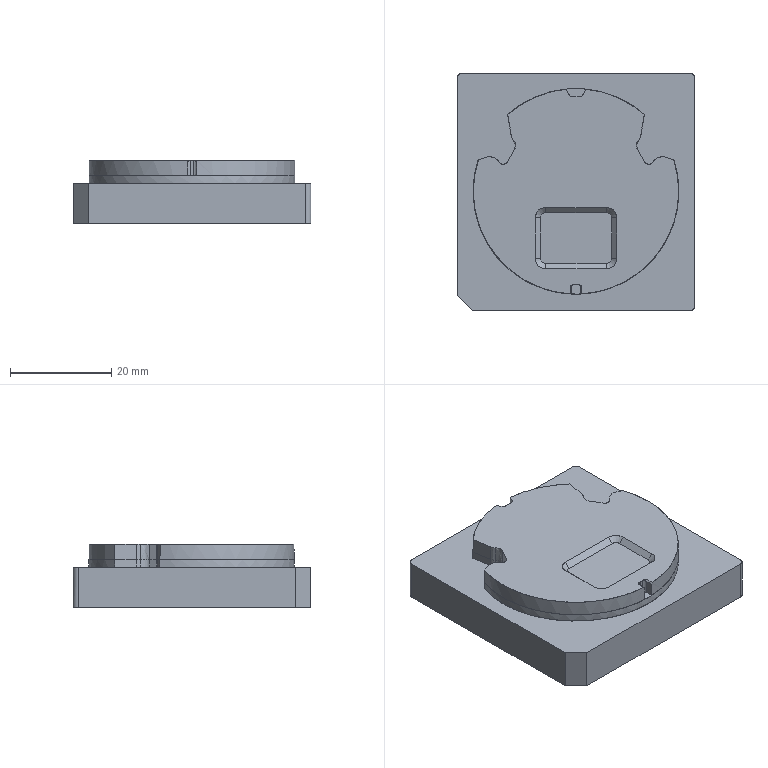NC program | PowerMill | posted with a generic post | part box 47 x 47 x 12.511 mm
Lines 10945 to 11810 of 232111:
N11042 M6
N11043 S22000 M03
N11044 G00 G90 X0.0 Y0.0
N11045 G43 Z9.8015 H27
N11046
N11047 G05 P10000 R4
N11048 X0.1631 Y19.5648
N11049 Z0.9432
N11050 G01 Z-0.2568 F1200.0
N11051 X0.1632 Y19.551 F2000.0
N11052 G03 X0.2878 Y19.4281 I0.1237 J0.0009
N11053 G01 X0.8947 Y19.4324
N11054 X0.9109 Y19.4372
N11055 X0.9228 Y19.4426
N11056 X0.9327 Y19.451
N11057 X0.9439 Y19.4635
N11058 X1.2092 Y20.0106
N11059 X0.163 Y19.5648 Z-0.3045
N11060 X0.1631 Y19.551
N11061 G03 X0.2877 Y19.4281 I0.1237 J0.0009
N11062 G01 X0.8947 Y19.4324
N11063 X0.9109 Y19.4372
N11064 X0.9228 Y19.4426
N11065 X0.9327 Y19.451
N11066 X0.9439 Y19.4635
N11067 X1.2092 Y20.0108
N11068 X0.1629 Y19.5648 Z-0.3523
N11069 X0.163 Y19.551
N11070 G03 X0.2876 Y19.4281 I0.1237 J0.0009
N11071 G01 X0.8947 Y19.4324
N11072 X0.9109 Y19.4372
N11073 X0.9228 Y19.4426
N11074 X0.9327 Y19.451
N11075 X0.9439 Y19.4635
N11076 X1.2093 Y20.0109
N11077 X0.1628 Y19.5648 Z-0.4001
N11078 X0.1629 Y19.551
N11079 G03 X0.2875 Y19.4281 I0.1237 J0.0009
N11080 G01 X0.8947 Y19.4324
N11081 X0.9109 Y19.4372
N11082 X0.9228 Y19.4426
N11083 X0.9327 Y19.451
N11084 X0.9439 Y19.4635
N11085 X1.2094 Y20.0111
N11086 X0.1626 Y19.5648 Z-0.4478
N11087 X0.1627 Y19.551
N11088 G03 X0.2874 Y19.4281 I0.1238 J0.0009
N11089 G01 X0.8947 Y19.4324
N11090 X0.9109 Y19.4372
N11091 X0.9228 Y19.4426
N11092 X0.9327 Y19.451
N11093 X0.9439 Y19.4635
N11094 X1.2094 Y20.0112
N11095 X0.1625 Y19.5648 Z-0.4956
N11096 X0.1626 Y19.551
N11097 G03 X0.2872 Y19.4281 I0.1238 J0.0009
N11098 G01 X0.8947 Y19.4324
N11099 X0.9109 Y19.4372
N11100 X0.9228 Y19.4426
N11101 X0.9327 Y19.451
N11102 X0.9439 Y19.4635
N11103 X1.2095 Y20.0113
N11104 X0.1624 Y19.5648 Z-0.5433
N11105 X0.1625 Y19.551
N11106 G03 X0.2871 Y19.4281 I0.1238 J0.0009
N11107 G01 X0.8947 Y19.4324
N11108 X0.9109 Y19.4372
N11109 X0.9228 Y19.4426
N11110 X0.9327 Y19.451
N11111 X0.9439 Y19.4635
N11112 X1.2096 Y20.0115
N11113 X0.1623 Y19.5648 Z-0.5911
N11114 X0.1624 Y19.551
N11115 G03 X0.287 Y19.4281 I0.1237 J0.0009
N11116 G01 X0.8947 Y19.4324
N11117 X0.9109 Y19.4372
N11118 X0.9228 Y19.4426
N11119 X0.9327 Y19.451
N11120 X0.9439 Y19.4635
N11121 X1.2096 Y20.0116
N11122 X0.1622 Y19.5648 Z-0.6389
N11123 X0.1623 Y19.551
N11124 G03 X0.2869 Y19.4281 I0.1237 J0.0009
N11125 G01 X0.8947 Y19.4324
N11126 X0.9109 Y19.4372
N11127 X0.9228 Y19.4426
N11128 X0.9327 Y19.451
N11129 X0.9439 Y19.4635
N11130 X1.2097 Y20.0117
N11131 X0.1621 Y19.5648 Z-0.6866
N11132 X0.1622 Y19.551
N11133 G03 X0.2868 Y19.4281 I0.1237 J0.0009
N11134 G01 X0.8947 Y19.4324
N11135 X0.9128 Y19.4377
N11136 X0.9226 Y19.4419
N11137 X0.9311 Y19.448
N11138 X0.9384 Y19.4547
N11139 X0.9439 Y19.4635
N11140 X1.2099 Y20.012
N11141 X0.162 Y19.5648 Z-0.7344
N11142 X0.1621 Y19.551
N11143 G03 X0.2867 Y19.4281 I0.1237 J0.0009
N11144 G01 X0.8947 Y19.4324
N11145 X0.911 Y19.4372
N11146 X0.9228 Y19.4426
N11147 X0.9327 Y19.4509
N11148 X0.9395 Y19.4585
N11149 X0.9435 Y19.4637
N11150 X0.9468 Y19.4694
N11151 X1.21 Y20.0121
N11152 X0.162 Y19.5648 Z-0.7821
N11153 X0.1621 Y19.551
N11154 G03 X0.2867 Y19.4281 I0.1237 J0.0009
N11155 G01 X0.8946 Y19.4324
N11156 X0.911 Y19.4372
N11157 X0.9228 Y19.4426
N11158 X0.9327 Y19.4509
N11159 X0.9439 Y19.4633
N11160 X0.9508 Y19.4774
N11161 X1.2101 Y20.0122
N11162 X0.1619 Y19.5648 Z-0.8299
N11163 X0.162 Y19.551
N11164 G03 X0.2867 Y19.4281 I0.1238 J0.0009
N11165 G01 X0.8946 Y19.4324
N11166 X0.911 Y19.4372
N11167 X0.9228 Y19.4426
N11168 X0.9327 Y19.4509
N11169 X0.9439 Y19.4633
N11170 X0.9553 Y19.4867
N11171 X1.2102 Y20.0123
N11172 X0.1619 Y19.5648 Z-0.8777
N11173 X0.162 Y19.551
N11174 G03 X0.2867 Y19.4281 I0.1238 J0.0009
N11175 G01 X0.8946 Y19.4324
N11176 X0.911 Y19.4372
N11177 X0.9228 Y19.4426
N11178 X0.9327 Y19.4509
N11179 X0.9439 Y19.4633
N11180 X0.9601 Y19.4965
N11181 X1.2103 Y20.0124
N11182 X0.1619 Y19.5648 Z-0.9254
N11183 X0.162 Y19.551
N11184 G03 X0.2866 Y19.4281 I0.1238 J0.0009
N11185 G01 X0.8946 Y19.4324
N11186 X0.911 Y19.4372
N11187 X0.9228 Y19.4425
N11188 X0.9327 Y19.4509
N11189 X0.9438 Y19.4633
N11190 X0.965 Y19.5063
N11191 X1.2104 Y20.0125
N11192 X0.1619 Y19.5648 Z-0.9732
N11193 X0.162 Y19.551
N11194 G03 X0.2866 Y19.4281 I0.1238 J0.0009
N11195 G01 X0.8946 Y19.4324
N11196 X0.911 Y19.4372
N11197 X0.9228 Y19.4425
N11198 X0.9327 Y19.4509
N11199 X0.9438 Y19.4633
N11200 X0.97 Y19.5167
N11201 X1.2105 Y20.0125
N11202 X0.1619 Y19.5648 Z-1.021
N11203 X0.162 Y19.551
N11204 G03 X0.2866 Y19.4281 I0.1237 J0.0009
N11205 G01 X0.8946 Y19.4324
N11206 X0.911 Y19.4372
N11207 X0.9228 Y19.4425
N11208 X0.9327 Y19.4509
N11209 X0.9438 Y19.4633
N11210 X0.9752 Y19.5272
N11211 X1.2106 Y20.0126
N11212 X0.1619 Y19.5648 Z-1.0687
N11213 X0.162 Y19.551
N11214 G03 X0.2866 Y19.4281 I0.1237 J0.0009
N11215 G01 X0.8946 Y19.4324
N11216 X0.911 Y19.4372
N11217 X0.9228 Y19.4425
N11218 X0.9327 Y19.4509
N11219 X0.9438 Y19.4633
N11220 X0.9806 Y19.5382
N11221 X1.2107 Y20.0127
N11222 X0.1619 Y19.5648 Z-1.1165
N11223 X0.162 Y19.551
N11224 G03 X0.2866 Y19.4281 I0.1237 J0.0009
N11225 G01 X0.8946 Y19.4324
N11226 X0.911 Y19.4372
N11227 X0.9228 Y19.4425
N11228 X0.9327 Y19.4509
N11229 X0.9438 Y19.4633
N11230 X0.9861 Y19.5494
N11231 X1.2108 Y20.0128
N11232 X0.1619 Y19.5648 Z-1.1643
N11233 X0.162 Y19.551
N11234 G03 X0.2866 Y19.4281 I0.1237 J0.0009
N11235 G01 X0.8946 Y19.4324
N11236 X0.911 Y19.4372
N11237 X0.9228 Y19.4425
N11238 X0.9327 Y19.4509
N11239 X0.9438 Y19.4633
N11240 X0.9918 Y19.5612
N11241 X1.2109 Y20.0129
N11242 X0.1619 Y19.5648 Z-1.2134
N11243 X0.162 Y19.551
N11244 G03 X0.2866 Y19.4281 I0.1237 J0.0009
N11245 G01 X0.8946 Y19.4324
N11246 X0.911 Y19.4372
N11247 X0.9228 Y19.4425
N11248 X0.9327 Y19.4509
N11249 X0.9438 Y19.4633
N11250 X0.9977 Y19.5732
N11251 X1.2109 Y20.0129
N11252 X0.1619 Y19.5648 Z-1.2626
N11253 X0.162 Y19.551
N11254 G03 X0.2866 Y19.4281 I0.1237 J0.0009
N11255 G01 X0.8946 Y19.4324
N11256 X0.911 Y19.4372
N11257 X0.9228 Y19.4425
N11258 X0.9327 Y19.4509
N11259 X0.9438 Y19.4633
N11260 X1.0039 Y19.5858
N11261 X1.2109 Y20.0128
N11262 X0.1618 Y19.5648 Z-1.3117
N11263 X0.1619 Y19.551
N11264 G03 X0.2866 Y19.4281 I0.1238 J0.0009
N11265 G01 X0.8946 Y19.4324
N11266 X0.911 Y19.4372
N11267 X0.9228 Y19.4425
N11268 X0.9327 Y19.4509
N11269 X0.9438 Y19.4633
N11270 X1.0102 Y19.5987
N11271 X1.211 Y20.0128
N11272 X0.1618 Y19.5648 Z-1.3609
N11273 X0.1619 Y19.551
N11274 G03 X0.2865 Y19.4281 I0.1238 J0.0009
N11275 G01 X0.8946 Y19.4324
N11276 X0.911 Y19.4372
N11277 X0.9228 Y19.4425
N11278 X0.9327 Y19.4509
N11279 X0.9438 Y19.4633
N11280 X1.0168 Y19.6121
N11281 X1.211 Y20.0128
N11282 X0.1619 Y19.5648 Z-1.4101
N11283 X0.162 Y19.551
N11284 G03 X0.2867 Y19.4281 I0.1238 J0.0009
N11285 G01 X0.8946 Y19.4324
N11286 X0.9109 Y19.4372
N11287 X0.9228 Y19.4425
N11288 X0.9327 Y19.4509
N11289 X0.9438 Y19.4633
N11290 X1.0236 Y19.6261
N11291 X1.211 Y20.0126
N11292 X0.1621 Y19.5648 Z-1.4592
N11293 X0.1622 Y19.551
N11294 G03 X0.2868 Y19.4281 I0.1237 J0.0009
N11295 G01 X0.8946 Y19.4324
N11296 X0.9109 Y19.4372
N11297 X0.9228 Y19.4425
N11298 X0.9327 Y19.4509
N11299 X0.9438 Y19.4633
N11300 X1.0307 Y19.6405
N11301 X1.211 Y20.0125
N11302 X0.1617 Y19.5648 Z-1.5084
N11303 X0.1618 Y19.551
N11304 G03 X0.2864 Y19.4281 I0.1237 J0.0009
N11305 G01 X0.8946 Y19.4324
N11306 X0.9109 Y19.4372
N11307 X0.9228 Y19.4425
N11308 X0.9327 Y19.4509
N11309 X0.9438 Y19.4633
N11310 X1.038 Y19.6556
N11311 X1.211 Y20.0124
N11312 X0.1622 Y19.5648 Z-1.5576
N11313 X0.1623 Y19.551
N11314 G03 X0.2869 Y19.4281 I0.1237 J0.0009
N11315 G01 X0.8946 Y19.4324
N11316 X0.9109 Y19.4372
N11317 X0.9228 Y19.4425
N11318 X0.9327 Y19.4509
N11319 X0.9438 Y19.4634
N11320 X1.0456 Y19.6712
N11321 X1.2111 Y20.0124
N11322 X0.1622 Y19.5648 Z-1.6067
N11323 X0.1623 Y19.551
N11324 G03 X0.2869 Y19.4281 I0.1237 J0.0009
N11325 G01 X0.8946 Y19.4324
N11326 X0.9109 Y19.4372
N11327 X0.9228 Y19.4425
N11328 X0.9327 Y19.4509
N11329 X0.9438 Y19.4634
N11330 X1.0535 Y19.6872
N11331 X1.2111 Y20.0124
N11332 X0.1622 Y19.5648 Z-1.6559
N11333 X0.1623 Y19.551
N11334 G03 X0.2869 Y19.4281 I0.1237 J0.0009
N11335 G01 X0.8946 Y19.4324
N11336 X0.9109 Y19.4372
N11337 X0.9228 Y19.4425
N11338 X0.9327 Y19.4509
N11339 X0.9438 Y19.4634
N11340 X1.0614 Y19.7035
N11341 X1.2111 Y20.0123
N11342 X0.1622 Y19.5648 Z-1.7051
N11343 X0.1623 Y19.551
N11344 G03 X0.2869 Y19.4281 I0.1237 J0.0009
N11345 G01 X0.8946 Y19.4324
N11346 X0.9109 Y19.4372
N11347 X0.9228 Y19.4425
N11348 X0.9327 Y19.4509
N11349 X0.9438 Y19.4634
N11350 X1.0697 Y19.7205
N11351 X1.2112 Y20.0123
N11352 X0.1621 Y19.5648 Z-1.7542
N11353 X0.1622 Y19.551
N11354 G03 X0.2869 Y19.4281 I0.1238 J0.0009
N11355 G01 X0.8946 Y19.4324
N11356 X0.9109 Y19.4372
N11357 X0.9228 Y19.4425
N11358 X0.9327 Y19.4509
N11359 X0.9438 Y19.4634
N11360 X1.0782 Y19.738
N11361 X1.2112 Y20.0123
N11362 X0.1621 Y19.5648 Z-1.8034
N11363 X0.1622 Y19.551
N11364 G03 X0.2868 Y19.4281 I0.1238 J0.0009
N11365 G01 X0.8946 Y19.4324
N11366 X0.9109 Y19.4372
N11367 X0.9228 Y19.4425
N11368 X0.9327 Y19.4509
N11369 X0.9438 Y19.4634
N11370 X1.0872 Y19.7563
N11371 X1.2113 Y20.0122
N11372 X0.1621 Y19.5648 Z-1.8526
N11373 X0.1622 Y19.551
N11374 G03 X0.2868 Y19.4281 I0.1238 J0.0009
N11375 G01 X0.8946 Y19.4324
N11376 X0.9109 Y19.4372
N11377 X0.9227 Y19.4425
N11378 X0.9327 Y19.4509
N11379 X0.9438 Y19.4634
N11380 X1.0964 Y19.7752
N11381 X1.2113 Y20.0122
N11382 X0.1621 Y19.5648 Z-1.9017
N11383 X0.1622 Y19.551
N11384 G03 X0.2868 Y19.4281 I0.1238 J0.0009
N11385 G01 X0.8946 Y19.4324
N11386 X0.9109 Y19.4372
N11387 X0.9227 Y19.4425
N11388 X0.9327 Y19.4509
N11389 X0.9438 Y19.4634
N11390 X1.1061 Y19.795
N11391 X1.2114 Y20.0122
N11392 X0.1621 Y19.5648 Z-1.9509
N11393 X0.1622 Y19.551
N11394 G03 X0.2868 Y19.4281 I0.1238 J0.0009
N11395 G01 X0.8946 Y19.4324
N11396 X0.9109 Y19.4372
N11397 X0.9227 Y19.4425
N11398 X0.9327 Y19.4509
N11399 X0.9438 Y19.4634
N11400 X1.116 Y19.8154
N11401 X1.2114 Y20.0122
N11402 X0.1621 Y19.5648 Z-2.0
N11403 X0.1622 Y19.551
N11404 G03 X0.2868 Y19.4281 I0.1237 J0.0009
N11405 G01 X0.8946 Y19.4324
N11406 X0.9109 Y19.4372
N11407 X0.9227 Y19.4425
N11408 X0.9327 Y19.4509
N11409 X0.9438 Y19.4634
N11410 X1.1265 Y19.8369
N11411 X1.2114 Y20.0121
N11412 X0.1621 Y19.5648 Z-2.0492
N11413 X0.1622 Y19.551
N11414 G03 X0.2868 Y19.4281 I0.1237 J0.0009
N11415 G01 X0.8946 Y19.4324
N11416 X0.9109 Y19.4372
N11417 X0.9227 Y19.4425
N11418 X0.9327 Y19.4509
N11419 X0.9438 Y19.4634
N11420 X1.1373 Y19.8591
N11421 X1.2115 Y20.0121
N11422 X0.1621 Y19.5648 Z-2.0984
N11423 X0.1622 Y19.551
N11424 G03 X0.2868 Y19.4281 I0.1237 J0.0009
N11425 G01 X0.8946 Y19.4324
N11426 X0.9109 Y19.4372
N11427 X0.9227 Y19.4425
N11428 X0.9327 Y19.4509
N11429 X0.9438 Y19.4634
N11430 X1.1486 Y19.8823
N11431 X1.2115 Y20.0121
N11432 X0.1621 Y19.5648 Z-2.1475
N11433 X0.1622 Y19.551
N11434 G03 X0.2868 Y19.4281 I0.1237 J0.0009
N11435 G01 X0.8946 Y19.4324
N11436 X0.9109 Y19.4372
N11437 X0.9227 Y19.4425
N11438 X0.9327 Y19.4509
N11439 X0.9438 Y19.4634
N11440 X1.1604 Y19.9066
N11441 X1.2116 Y20.012
N11442 X0.1621 Y19.5648 Z-2.1967
N11443 X0.1622 Y19.551
N11444 G03 X0.2868 Y19.4281 I0.1237 J0.0009
N11445 G01 X0.8946 Y19.4324
N11446 X0.9109 Y19.4372
N11447 X0.9227 Y19.4425
N11448 X0.9326 Y19.4509
N11449 X0.9438 Y19.4634
N11450 X1.1728 Y19.9319
N11451 X1.2116 Y20.012
N11452 X0.1621 Y19.5648 Z-2.2459
N11453 Y19.551
N11454 G03 X0.2868 Y19.4281 I0.1238 J0.0009
N11455 G01 X0.8946 Y19.4324
N11456 X0.9109 Y19.4372
N11457 X0.9227 Y19.4425
N11458 X0.9326 Y19.4509
N11459 X0.9438 Y19.4634
N11460 X1.1857 Y19.9585
N11461 X1.2116 Y20.012
N11462 X0.162 Y19.5648 Z-2.295
N11463 X0.1621 Y19.551
N11464 G03 X0.2868 Y19.4281 I0.1238 J0.0009
N11465 G01 X0.8946 Y19.4324
N11466 X0.9109 Y19.4372
N11467 X0.9227 Y19.4425
N11468 X0.9326 Y19.4509
N11469 X0.9438 Y19.4634
N11470 X1.1992 Y19.9863
N11471 X1.2117 Y20.012
N11472 X0.162 Y19.5648 Z-2.3442
N11473 X0.1621 Y19.551
N11474 G03 X0.2867 Y19.4281 I0.1238 J0.0009
N11475 G01 X0.8946 Y19.4324
N11476 X0.9109 Y19.4372
N11477 X0.9227 Y19.4425
N11478 X0.9326 Y19.4509
N11479 X0.9438 Y19.4634
N11480 X1.2117 Y20.0119
N11481 X0.162 Y19.5648 Z-2.3934
N11482 X0.1621 Y19.551
N11483 G03 X0.2867 Y19.4281 I0.1238 J0.0009
N11484 G01 X0.8946 Y19.4324
N11485 X0.9109 Y19.4372
N11486 X0.9227 Y19.4425
N11487 X0.9326 Y19.4509
N11488 X0.9438 Y19.4634
N11489 X1.2117 Y20.0119
N11490 X0.162 Y19.5648 Z-2.4425
N11491 X0.1621 Y19.551
N11492 G03 X0.2867 Y19.4281 I0.1238 J0.0009
N11493 G01 X0.8946 Y19.4324
N11494 X0.9109 Y19.4372
N11495 X0.9227 Y19.4425
N11496 X0.9326 Y19.4509
N11497 X0.9438 Y19.4634
N11498 X1.2116 Y20.012
N11499 X0.162 Y19.5648 Z-2.4917
N11500 X0.1621 Y19.551
N11501 G03 X0.2867 Y19.4281 I0.1237 J0.0009
N11502 G01 X0.8946 Y19.4324
N11503 X0.9109 Y19.4372
N11504 X0.9227 Y19.4425
N11505 X0.9326 Y19.4509
N11506 X0.9438 Y19.4634
N11507 X1.2116 Y20.012
N11508 X0.162 Y19.5647 Z-2.5408
N11509 X0.1621 Y19.551
N11510 G03 X0.2867 Y19.4281 I0.1237 J0.0009
N11511 G01 X0.8946 Y19.4324
N11512 X0.9109 Y19.4372
N11513 X0.9227 Y19.4425
N11514 X0.9326 Y19.4509
N11515 X0.9438 Y19.4634
N11516 X1.2116 Y20.012
N11517 X0.162 Y19.5647 Z-2.59
N11518 X0.1621 Y19.551
N11519 G03 X0.2867 Y19.4281 I0.1237 J0.0009
N11520 G01 X0.8946 Y19.4324
N11521 X0.9109 Y19.4372
N11522 X0.9227 Y19.4425
N11523 X0.9326 Y19.4509
N11524 X0.9438 Y19.4634
N11525 X1.2115 Y20.012
N11526 X0.162 Y19.5647 Z-2.6392
N11527 X0.1621 Y19.551
N11528 G03 X0.2867 Y19.4281 I0.1237 J0.0009
N11529 G01 X0.8946 Y19.4324
N11530 X0.9109 Y19.4372
N11531 X0.9227 Y19.4425
N11532 X0.9326 Y19.4509
N11533 X0.9438 Y19.4634
N11534 X1.2115 Y20.012
N11535 X0.162 Y19.5647 Z-2.6883
N11536 X0.1621 Y19.551
N11537 G03 X0.2867 Y19.4281 I0.1237 J0.0009
N11538 G01 X0.8946 Y19.4324
N11539 X0.9108 Y19.4372
N11540 X0.9227 Y19.4425
N11541 X0.9326 Y19.4509
N11542 X0.9438 Y19.4634
N11543 X1.2114 Y20.012
N11544 X0.162 Y19.5647 Z-2.7375
N11545 X0.1621 Y19.551
N11546 G03 X0.2867 Y19.4281 I0.1237 J0.0009
N11547 G01 X0.8946 Y19.4324
N11548 X0.9108 Y19.4372
N11549 X0.9227 Y19.4425
N11550 X0.9326 Y19.4509
N11551 X0.9438 Y19.4634
N11552 X1.2114 Y20.012
N11553 X0.1619 Y19.5647 Z-2.7867
N11554 X0.162 Y19.551
N11555 G03 X0.2867 Y19.4281 I0.1238 J0.0009
N11556 G01 X0.8946 Y19.4324
N11557 X0.9108 Y19.4372
N11558 X0.9227 Y19.4425
N11559 X0.9326 Y19.4509
N11560 X0.9438 Y19.4634
N11561 X1.2114 Y20.012
N11562 X0.1619 Y19.5647 Z-2.8358
N11563 X0.162 Y19.551
N11564 G03 X0.2866 Y19.4281 I0.1238 J0.0009
N11565 G01 X0.8946 Y19.4324
N11566 X0.9108 Y19.4372
N11567 X0.9227 Y19.4425
N11568 X0.9326 Y19.4509
N11569 X0.9438 Y19.4634
N11570 X1.2113 Y20.0121
N11571 X0.1619 Y19.5647 Z-2.885
N11572 X0.162 Y19.551
N11573 G03 X0.2866 Y19.4281 I0.1238 J0.0009
N11574 G01 X0.8946 Y19.4324
N11575 X0.9108 Y19.4372
N11576 X0.9227 Y19.4425
N11577 X0.9326 Y19.4509
N11578 X0.9438 Y19.4634
N11579 X1.2113 Y20.0121
N11580 X0.1619 Y19.5647 Z-2.9342
N11581 X0.162 Y19.551
N11582 G03 X0.2866 Y19.4281 I0.1238 J0.0009
N11583 G01 X0.8946 Y19.4324
N11584 X0.9108 Y19.4372
N11585 X0.9227 Y19.4425
N11586 X0.9326 Y19.4509
N11587 X0.9438 Y19.4634
N11588 X1.2112 Y20.0121
N11589 X0.1619 Y19.5647 Z-2.9833
N11590 X0.162 Y19.551
N11591 G03 X0.2866 Y19.4281 I0.1238 J0.0009
N11592 G01 X0.8946 Y19.4324
N11593 X0.9108 Y19.4372
N11594 X0.9227 Y19.4425
N11595 X0.9326 Y19.4509
N11596 X0.9438 Y19.4634
N11597 X1.2112 Y20.0121
N11598 X0.1619 Y19.5647 Z-3.0325
N11599 X0.162 Y19.551
N11600 G03 X0.2866 Y19.4281 I0.1237 J0.0009
N11601 G01 X0.8946 Y19.4324
N11602 X0.9108 Y19.4372
N11603 X0.9227 Y19.4425
N11604 X0.9326 Y19.4509
N11605 X0.9438 Y19.4634
N11606 X1.2112 Y20.0121
N11607 X0.1619 Y19.5647 Z-3.0817
N11608 X0.162 Y19.551
N11609 G03 X0.2866 Y19.4281 I0.1237 J0.0009
N11610 G01 X0.8946 Y19.4324
N11611 X0.9108 Y19.4372
N11612 X0.9227 Y19.4425
N11613 X0.9326 Y19.4509
N11614 X0.9438 Y19.4634
N11615 X1.2111 Y20.0121
N11616 X0.1619 Y19.5647 Z-3.1308
N11617 X0.162 Y19.551
N11618 G03 X0.2866 Y19.4281 I0.1237 J0.0009
N11619 G01 X0.8946 Y19.4324
N11620 X0.9108 Y19.4372
N11621 X0.9227 Y19.4425
N11622 X0.9326 Y19.4509
N11623 X0.9438 Y19.4634
N11624 X1.2111 Y20.0121
N11625 X0.1619 Y19.5647 Z-3.18
N11626 X0.162 Y19.551
N11627 G03 X0.2866 Y19.4281 I0.1237 J0.0009
N11628 G01 X0.8946 Y19.4324
N11629 X0.9108 Y19.4372
N11630 X0.9227 Y19.4425
N11631 X0.9326 Y19.4509
N11632 X0.9438 Y19.4634
N11633 X1.211 Y20.0121
N11634 G00 Z3.9432
N11635 G01 X-1.1458 Y20.1841 F10000.0
N11636 G00 Z0.9432
N11637 G01 Z-0.2568 F1200.0
N11638 X-1.1581 Y20.1781 F2000.0
N11639 G03 X-1.2145 Y20.0124 I0.0546 J-0.111
N11640 G01 X-0.9443 Y19.4636
N11641 X-0.9265 Y19.4436
N11642 X-0.9096 Y19.4328
N11643 X-0.8446 Y19.4202
N11644 X-0.2641 Y19.4243
N11645 X-1.1457 Y20.1842 Z-0.3045
N11646 X-1.158 Y20.1781
N11647 G03 X-1.2144 Y20.0124 I0.0546 J-0.111
N11648 G01 X-0.9443 Y19.4636
N11649 X-0.9265 Y19.4436
N11650 X-0.9096 Y19.4328
N11651 X-0.8446 Y19.4202
N11652 X-0.264 Y19.4243
N11653 X-1.1456 Y20.1842 Z-0.3523
N11654 X-1.158 Y20.1781
N11655 G03 X-1.2144 Y20.0124 I0.0547 J-0.111
N11656 G01 X-0.9443 Y19.4636
N11657 X-0.9265 Y19.4436
N11658 X-0.9096 Y19.4328
N11659 X-0.8446 Y19.4202
N11660 X-0.264 Y19.4243
N11661 X-1.1456 Y20.1842 Z-0.4001
N11662 X-1.1579 Y20.1781
N11663 G03 X-1.2143 Y20.0125 I0.0546 J-0.111
N11664 G01 X-0.9443 Y19.4636
N11665 X-0.9265 Y19.4436
N11666 X-0.9096 Y19.4328
N11667 X-0.8446 Y19.4202
N11668 X-0.264 Y19.4243
N11669 X-1.1455 Y20.1842 Z-0.4478
N11670 X-1.1578 Y20.1781
N11671 G03 X-1.2143 Y20.0125 I0.0546 J-0.111
N11672 G01 X-0.9443 Y19.4636
N11673 X-0.9265 Y19.4436
N11674 X-0.9096 Y19.4328
N11675 X-0.8446 Y19.4202
N11676 X-0.264 Y19.4243
N11677 X-1.1454 Y20.1842 Z-0.4956
N11678 X-1.1578 Y20.1781
N11679 G03 X-1.2142 Y20.0125 I0.0546 J-0.111
N11680 G01 X-0.9443 Y19.4636
N11681 X-0.9265 Y19.4436
N11682 X-0.9096 Y19.4328
N11683 X-0.8446 Y19.4202
N11684 X-0.264 Y19.4243
N11685 X-1.1454 Y20.1842 Z-0.5433
N11686 X-1.1577 Y20.1782
N11687 G03 X-1.2142 Y20.0125 I0.0546 J-0.1111
N11688 G01 X-0.9443 Y19.4636
N11689 X-0.9264 Y19.4436
N11690 X-0.9096 Y19.4328
N11691 X-0.8446 Y19.4202
N11692 X-0.264 Y19.4243
N11693 X-1.1453 Y20.1842 Z-0.5911
N11694 X-1.1576 Y20.1782
N11695 G03 X-1.2141 Y20.0125 I0.0546 J-0.1111
N11696 G01 X-0.9443 Y19.4636
N11697 X-0.9264 Y19.4436
N11698 X-0.9096 Y19.4328
N11699 X-0.8446 Y19.4202
N11700 X-0.264 Y19.4243
N11701 X-1.1452 Y20.1843 Z-0.6389
N11702 X-1.1576 Y20.1782
N11703 G03 X-1.214 Y20.0125 I0.0546 J-0.1111
N11704 G01 X-0.9443 Y19.4637
N11705 X-0.9264 Y19.4436
N11706 X-0.9096 Y19.4328
N11707 X-0.8446 Y19.4202
N11708 X-0.264 Y19.4243
N11709 X-1.1451 Y20.1843 Z-0.6866
N11710 X-1.1575 Y20.1782
N11711 G03 X-1.214 Y20.0126 I0.0546 J-0.1111
N11712 G01 X-0.9443 Y19.4637
N11713 X-0.9264 Y19.4436
N11714 X-0.9096 Y19.4328
N11715 X-0.8446 Y19.4202
N11716 X-0.2639 Y19.4243
N11717 X-1.1451 Y20.1843 Z-0.7344
N11718 X-1.1574 Y20.1782
N11719 G03 X-1.2139 Y20.0126 I0.0545 J-0.1111
N11720 G01 X-0.9443 Y19.4637
N11721 X-0.9264 Y19.4436
N11722 X-0.9096 Y19.4328
N11723 X-0.8446 Y19.4202
N11724 X-0.2639 Y19.4243
N11725 X-1.145 Y20.1843 Z-0.7821
N11726 X-1.1574 Y20.1782
N11727 G03 X-1.2139 Y20.0126 I0.0546 J-0.1111
N11728 G01 X-0.9443 Y19.4637
N11729 X-0.9264 Y19.4436
N11730 X-0.9096 Y19.4328
N11731 X-0.8446 Y19.4202
N11732 X-0.2639 Y19.4243
N11733 X-1.1449 Y20.1843 Z-0.8299
N11734 X-1.1573 Y20.1782
N11735 G03 X-1.2138 Y20.0126 I0.0546 J-0.111
N11736 G01 X-0.9443 Y19.4637
N11737 X-0.9264 Y19.4436
N11738 X-0.9095 Y19.4328
N11739 X-0.8446 Y19.4202
N11740 X-0.2639 Y19.4243
N11741 X-1.1449 Y20.1843 Z-0.8777
N11742 X-1.1572 Y20.1783
N11743 G03 X-1.2138 Y20.0126 I0.0545 J-0.1111
N11744 G01 X-0.9443 Y19.4637
N11745 X-0.9264 Y19.4436
N11746 X-0.9095 Y19.4328
N11747 X-0.8446 Y19.4202
N11748 X-0.2639 Y19.4243
N11749 X-1.1448 Y20.1843 Z-0.9254
N11750 X-1.1571 Y20.1783
N11751 G03 X-1.2137 Y20.0127 I0.0545 J-0.1111
N11752 G01 X-0.9443 Y19.4637
N11753 X-0.9264 Y19.4436
N11754 X-0.9095 Y19.4328
N11755 X-0.8446 Y19.4202
N11756 X-0.2639 Y19.4243
N11757 X-1.1447 Y20.1843 Z-0.9732
N11758 X-1.1571 Y20.1783
N11759 G03 X-1.2137 Y20.0127 I0.0545 J-0.1111
N11760 G01 X-0.9443 Y19.4637
N11761 X-0.9264 Y19.4436
N11762 X-0.9095 Y19.4328
N11763 X-0.8446 Y19.4202
N11764 X-0.2639 Y19.4243
N11765 X-1.1447 Y20.1844 Z-1.021
N11766 X-1.157 Y20.1783
N11767 G03 X-1.2136 Y20.0127 I0.0545 J-0.1111
N11768 G01 X-0.9443 Y19.4637
N11769 X-0.9264 Y19.4436
N11770 X-0.9095 Y19.4328
N11771 X-0.8446 Y19.4202
N11772 X-0.2638 Y19.4243
N11773 X-1.1446 Y20.1844 Z-1.0687
N11774 X-1.157 Y20.1783
N11775 G03 X-1.2136 Y20.0127 I0.0545 J-0.1111
N11776 G01 X-0.9443 Y19.4637
N11777 X-0.9264 Y19.4436
N11778 X-0.9095 Y19.4328
N11779 X-0.8446 Y19.4202
N11780 X-0.2638 Y19.4243
N11781 X-1.1446 Y20.1844 Z-1.1165
N11782 X-1.1569 Y20.1783
N11783 G03 X-1.2135 Y20.0127 I0.0545 J-0.1111
N11784 G01 X-0.9443 Y19.4637
N11785 X-0.9264 Y19.4436
N11786 X-0.9095 Y19.4328
N11787 X-0.8446 Y19.4202
N11788 X-0.2638 Y19.4243
N11789 X-1.1445 Y20.1844 Z-1.1643
N11790 X-1.1569 Y20.1783
N11791 G03 X-1.2135 Y20.0127 I0.0545 J-0.1111
N11792 G01 X-0.9443 Y19.4637
N11793 X-0.9264 Y19.4436
N11794 X-0.9095 Y19.4328
N11795 X-0.8446 Y19.4202
N11796 X-0.2638 Y19.4243
N11797 X-1.1445 Y20.1844 Z-1.2134
N11798 X-1.1568 Y20.1783
N11799 G03 X-1.2135 Y20.0128 I0.0545 J-0.1111
N11800 G01 X-0.9443 Y19.4637
N11801 X-0.9264 Y19.4436
N11802 X-0.9095 Y19.4328
N11803 X-0.8446 Y19.4202
N11804 X-0.2638 Y19.4243
N11805 X-1.1444 Y20.1844 Z-1.2626
N11806 X-1.1567 Y20.1784
N11807 G03 X-1.2134 Y20.0128 I0.0544 J-0.1112
N11808 G01 X-0.9443 Y19.4637
N11809 X-0.9264 Y19.4436
N11810 X-0.9095 Y19.4328
N11811 X-0.8446 Y19.4202
N11812 X-0.2638 Y19.4243
N11813 X-1.1443 Y20.1844 Z-1.3117
N11814 X-1.1567 Y20.1784
N11815 G03 X-1.2134 Y20.0128 I0.0545 J-0.1112
N11816 G01 X-0.9443 Y19.4637
N11817 X-0.9264 Y19.4436
N11818 X-0.9095 Y19.4328
N11819 X-0.8446 Y19.4202
N11820 X-0.2638 Y19.4243
N11821 X-1.1443 Y20.1844 Z-1.3609
N11822 X-1.1566 Y20.1784
N11823 G03 X-1.2133 Y20.0128 I0.0544 J-0.1112
N11824 G01 X-0.9443 Y19.4637
N11825 X-0.9264 Y19.4436
N11826 X-0.9095 Y19.4328
N11827 X-0.8446 Y19.4202
N11828 X-0.2638 Y19.4243
N11829 X-1.1442 Y20.1843 Z-1.4101
N11830 X-1.1565 Y20.1783
N11831 G03 X-1.2132 Y20.0127 I0.0544 J-0.1112
N11832 G01 X-0.9443 Y19.4637
N11833 X-0.9264 Y19.4436
N11834 X-0.9095 Y19.4328
N11835 X-0.8446 Y19.4202
N11836 X-0.2639 Y19.4243
N11837 X-1.1441 Y20.1842 Z-1.4592
N11838 X-1.1564 Y20.1782
N11839 G03 X-1.2131 Y20.0126 I0.0544 J-0.1112
N11840 G01 X-0.9443 Y19.4637
N11841 X-0.9264 Y19.4436
N11842 X-0.9095 Y19.4328
N11843 X-0.8446 Y19.4202
N11844 X-0.264 Y19.4243
N11845 X-1.1439 Y20.1841 Z-1.5084
N11846 X-1.1563 Y20.1781
N11847 G03 X-1.213 Y20.0125 I0.0544 J-0.1112
N11848 G01 X-0.9443 Y19.4637
N11849 X-0.9264 Y19.4436
N11850 X-0.9095 Y19.4328
N11851 X-0.8446 Y19.4202
N11852 X-0.2641 Y19.4243
N11853 X-1.1438 Y20.184 Z-1.5576
N11854 X-1.1562 Y20.178
N11855 G03 X-1.2129 Y20.0124 I0.0544 J-0.1112
N11856 G01 X-0.9443 Y19.4637
N11857 X-0.9264 Y19.4436
N11858 X-0.9095 Y19.4328
N11859 X-0.8446 Y19.4202
N11860 X-0.2642 Y19.4243
N11861 X-1.1437 Y20.1839 Z-1.6067
N11862 X-1.1561 Y20.1779
N11863 G03 X-1.2128 Y20.0123 I0.0544 J-0.1112
N11864 G01 X-0.9443 Y19.4637
N11865 X-0.9264 Y19.4436
N11866 X-0.9095 Y19.4328
N11867 X-0.8446 Y19.4202
N11868 X-0.2643 Y19.4243
N11869 X-1.1436 Y20.1838 Z-1.6559
N11870 X-1.1559 Y20.1778
N11871 G03 X-1.2127 Y20.0122 I0.0544 J-0.1112
N11872 G01 X-0.9443 Y19.4637
N11873 X-0.9264 Y19.4436
N11874 X-0.9095 Y19.4328
N11875 X-0.8446 Y19.4202
N11876 X-0.2645 Y19.4243
N11877 X-1.1435 Y20.1837 Z-1.7051
N11878 X-1.1558 Y20.1777
N11879 G03 X-1.2126 Y20.0121 I0.0544 J-0.1112
N11880 G01 X-0.9443 Y19.4637
N11881 X-0.9264 Y19.4436
N11882 X-0.9095 Y19.4328
N11883 X-0.8445 Y19.4202
N11884 X-0.2646 Y19.4243
N11885 X-1.1434 Y20.1836 Z-1.7542
N11886 X-1.1557 Y20.1775
N11887 G03 X-1.2125 Y20.012 I0.0544 J-0.1111
N11888 G01 X-0.9443 Y19.4637
N11889 X-0.9264 Y19.4436
N11890 X-0.9095 Y19.4328
N11891 X-0.8445 Y19.4202
N11892 X-0.2647 Y19.4243
N11893 X-1.1433 Y20.1835 Z-1.8034
N11894 X-1.1556 Y20.1774
N11895 G03 X-1.2124 Y20.0119 I0.0544 J-0.1111
N11896 G01 X-0.9443 Y19.4637
N11897 X-0.9264 Y19.4436
N11898 X-0.9095 Y19.4328
N11899 X-0.8445 Y19.4202
N11900 X-0.2648 Y19.4243
N11901 X-1.1431 Y20.1834 Z-1.8526
N11902 X-1.1555 Y20.1773
N11903 G03 X-1.2123 Y20.0118 I0.0544 J-0.1111
N11904 G01 X-0.9443 Y19.4637
N11905 X-0.9264 Y19.4436
N11906 X-0.9095 Y19.4328
N11907 X-0.8445 Y19.4202